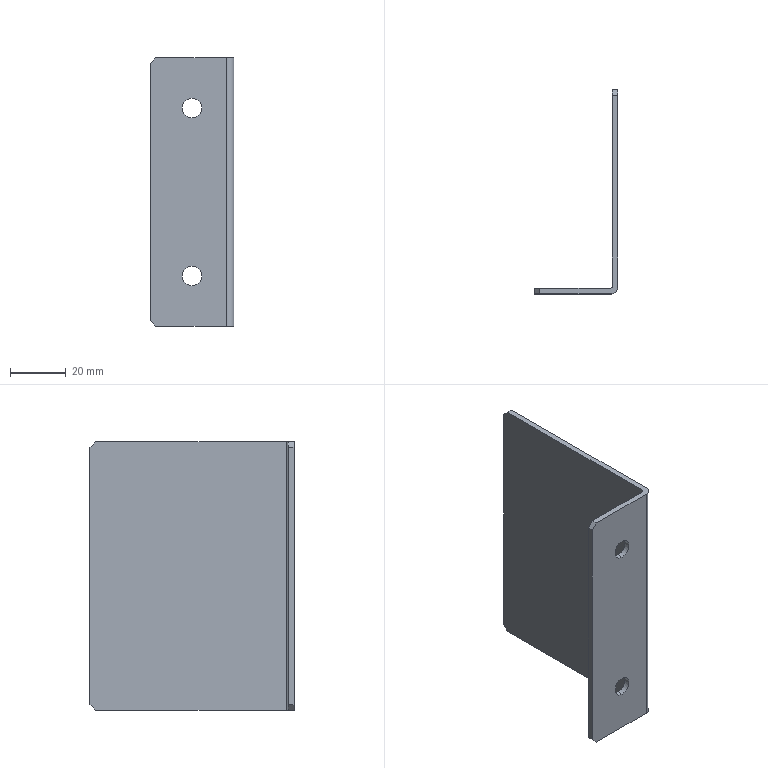Part | SolidWorks | features BaseBody 1 | 1 solid | 18 faces | box 30 x 73 x 96 mm | volume 19079 mm3 | plane 12 | cylinder 6 | commonest cylinder face diameters 7 x4 1.473 x1 5.473 x1
STEP:
#1=CARTESIAN_POINT('',(15.,0.,14.5));
#2=VERTEX_POINT('',#1);
#3=CARTESIAN_POINT('',(15.,0.,21.5));
#4=VERTEX_POINT('',#3);
#5=CARTESIAN_POINT('',(15.,0.,18.));
#6=DIRECTION('',(0.,1.,0.));
#7=DIRECTION('',(0.,0.,1.));
#8=AXIS2_PLACEMENT_3D('',#5,#6,#7);
#9=CIRCLE('',#8,3.5);
#10=EDGE_CURVE('',#2,#4,#9,.T.);
#11=ORIENTED_EDGE('',*,*,#10,.F.);
#12=CARTESIAN_POINT('',(15.,2.,14.5));
#13=VERTEX_POINT('',#12);
#14=CARTESIAN_POINT('',(15.,2.,14.5));
#15=DIRECTION('',(0.,1.,0.));
#16=VECTOR('',#15,1000.);
#17=LINE('',#14,#16);
#18=EDGE_CURVE('',#2,#13,#17,.T.);
#19=ORIENTED_EDGE('',*,*,#18,.T.);
#20=CARTESIAN_POINT('',(15.,2.,21.5));
#21=VERTEX_POINT('',#20);
#22=CARTESIAN_POINT('',(15.,2.,18.));
#23=DIRECTION('',(0.,1.,0.));
#24=DIRECTION('',(0.,0.,1.));
#25=AXIS2_PLACEMENT_3D('',#22,#23,#24);
#26=CIRCLE('',#25,3.5);
#27=EDGE_CURVE('',#13,#21,#26,.T.);
#28=ORIENTED_EDGE('',*,*,#27,.T.);
#29=CARTESIAN_POINT('',(15.,2.,21.5));
#30=DIRECTION('',(0.,1.,0.));
#31=VECTOR('',#30,1000.);
#32=LINE('',#29,#31);
#33=EDGE_CURVE('',#4,#21,#32,.T.);
#34=ORIENTED_EDGE('',*,*,#33,.F.);
#35=EDGE_LOOP('',(#11,#19,#28,#34));
#36=FACE_OUTER_BOUND('',#35,.T.);
#37=CARTESIAN_POINT('',(15.,2.,18.));
#38=DIRECTION('',(0.,1.,0.));
#39=DIRECTION('',(0.,0.,1.));
#40=AXIS2_PLACEMENT_3D('',#37,#38,#39);
#41=CYLINDRICAL_SURFACE('',#40,3.5);
#42=ADVANCED_FACE('',(#36),#41,.F.);
#43=CARTESIAN_POINT('',(15.,0.,74.5));
#44=VERTEX_POINT('',#43);
#45=CARTESIAN_POINT('',(15.,0.,81.5));
#46=VERTEX_POINT('',#45);
#47=CARTESIAN_POINT('',(15.,0.,78.));
#48=DIRECTION('',(0.,1.,0.));
#49=DIRECTION('',(0.,0.,1.));
#50=AXIS2_PLACEMENT_3D('',#47,#48,#49);
#51=CIRCLE('',#50,3.5);
#52=EDGE_CURVE('',#44,#46,#51,.T.);
#53=ORIENTED_EDGE('',*,*,#52,.F.);
#54=CARTESIAN_POINT('',(15.,2.,74.5));
#55=VERTEX_POINT('',#54);
#56=CARTESIAN_POINT('',(15.,2.,74.5));
#57=DIRECTION('',(0.,1.,0.));
#58=VECTOR('',#57,1000.);
#59=LINE('',#56,#58);
#60=EDGE_CURVE('',#44,#55,#59,.T.);
#61=ORIENTED_EDGE('',*,*,#60,.T.);
#62=CARTESIAN_POINT('',(15.,2.,81.5));
#63=VERTEX_POINT('',#62);
#64=CARTESIAN_POINT('',(15.,2.,78.));
#65=DIRECTION('',(0.,1.,0.));
#66=DIRECTION('',(0.,0.,1.));
#67=AXIS2_PLACEMENT_3D('',#64,#65,#66);
#68=CIRCLE('',#67,3.5);
#69=EDGE_CURVE('',#55,#63,#68,.T.);
#70=ORIENTED_EDGE('',*,*,#69,.T.);
#71=CARTESIAN_POINT('',(15.,2.,81.5));
#72=DIRECTION('',(0.,1.,0.));
#73=VECTOR('',#72,1000.);
#74=LINE('',#71,#73);
#75=EDGE_CURVE('',#46,#63,#74,.T.);
#76=ORIENTED_EDGE('',*,*,#75,.F.);
#77=EDGE_LOOP('',(#53,#61,#70,#76));
#78=FACE_OUTER_BOUND('',#77,.T.);
#79=CARTESIAN_POINT('',(15.,2.,78.));
#80=DIRECTION('',(0.,1.,0.));
#81=DIRECTION('',(0.,0.,1.));
#82=AXIS2_PLACEMENT_3D('',#79,#80,#81);
#83=CYLINDRICAL_SURFACE('',#82,3.5);
#84=ADVANCED_FACE('',(#78),#83,.F.);
#85=CARTESIAN_POINT('',(0.,0.,2.));
#86=VERTEX_POINT('',#85);
#87=CARTESIAN_POINT('',(2.,0.,0.));
#88=VERTEX_POINT('',#87);
#89=CARTESIAN_POINT('',(2.,0.,0.));
#90=DIRECTION('',(0.7071,0.,-0.7071));
#91=VECTOR('',#90,1000.);
#92=LINE('',#89,#91);
#93=EDGE_CURVE('',#86,#88,#92,.T.);
#94=ORIENTED_EDGE('',*,*,#93,.F.);
#95=CARTESIAN_POINT('',(0.,2.,2.));
#96=VERTEX_POINT('',#95);
#97=CARTESIAN_POINT('',(0.,0.,2.));
#98=DIRECTION('',(0.,-1.,0.));
#99=VECTOR('',#98,1000.);
#100=LINE('',#97,#99);
#101=EDGE_CURVE('',#96,#86,#100,.T.);
#102=ORIENTED_EDGE('',*,*,#101,.F.);
#103=CARTESIAN_POINT('',(2.,2.,0.));
#104=VERTEX_POINT('',#103);
#105=CARTESIAN_POINT('',(-47.,2.,49.));
#106=DIRECTION('',(-0.7071,0.,0.7071));
#107=VECTOR('',#106,1000.);
#108=LINE('',#105,#107);
#109=EDGE_CURVE('',#104,#96,#108,.T.);
#110=ORIENTED_EDGE('',*,*,#109,.F.);
#111=CARTESIAN_POINT('',(2.,2.,0.));
#112=DIRECTION('',(0.,1.,0.));
#113=VECTOR('',#112,1000.);
#114=LINE('',#111,#113);
#115=EDGE_CURVE('',#88,#104,#114,.T.);
#116=ORIENTED_EDGE('',*,*,#115,.F.);
#117=EDGE_LOOP('',(#94,#102,#110,#116));
#118=FACE_OUTER_BOUND('',#117,.T.);
#119=CARTESIAN_POINT('',(2.,2.737,0.));
#120=DIRECTION('',(-0.7071,0.,-0.7071));
#121=DIRECTION('',(-0.7071,0.,0.7071));
#122=AXIS2_PLACEMENT_3D('',#119,#120,#121);
#123=PLANE('',#122);
#124=ADVANCED_FACE('',(#118),#123,.T.);
#125=CARTESIAN_POINT('',(2.,0.,96.));
#126=VERTEX_POINT('',#125);
#127=CARTESIAN_POINT('',(0.,0.,94.));
#128=VERTEX_POINT('',#127);
#129=CARTESIAN_POINT('',(0.,0.,94.));
#130=DIRECTION('',(-0.7071,0.,-0.7071));
#131=VECTOR('',#130,1000.);
#132=LINE('',#129,#131);
#133=EDGE_CURVE('',#126,#128,#132,.T.);
#134=ORIENTED_EDGE('',*,*,#133,.F.);
#135=CARTESIAN_POINT('',(2.,2.,96.));
#136=VERTEX_POINT('',#135);
#137=CARTESIAN_POINT('',(2.,2.737,96.));
#138=DIRECTION('',(0.,-1.,0.));
#139=VECTOR('',#138,1000.);
#140=LINE('',#137,#139);
#141=EDGE_CURVE('',#136,#126,#140,.T.);
#142=ORIENTED_EDGE('',*,*,#141,.F.);
#143=CARTESIAN_POINT('',(0.,2.,94.));
#144=VERTEX_POINT('',#143);
#145=CARTESIAN_POINT('',(1.,2.,95.));
#146=DIRECTION('',(0.7071,0.,0.7071));
#147=VECTOR('',#146,1000.);
#148=LINE('',#145,#147);
#149=EDGE_CURVE('',#144,#136,#148,.T.);
#150=ORIENTED_EDGE('',*,*,#149,.F.);
#151=CARTESIAN_POINT('',(0.,0.,94.));
#152=DIRECTION('',(0.,1.,0.));
#153=VECTOR('',#152,1000.);
#154=LINE('',#151,#153);
#155=EDGE_CURVE('',#128,#144,#154,.T.);
#156=ORIENTED_EDGE('',*,*,#155,.F.);
#157=EDGE_LOOP('',(#134,#142,#150,#156));
#158=FACE_OUTER_BOUND('',#157,.T.);
#159=CARTESIAN_POINT('',(0.,0.,94.));
#160=DIRECTION('',(0.7071,0.,-0.7071));
#161=DIRECTION('',(0.,-1.,0.));
#162=AXIS2_PLACEMENT_3D('',#159,#160,#161);
#163=PLANE('',#162);
#164=ADVANCED_FACE('',(#158),#163,.F.);
#165=CARTESIAN_POINT('',(28.,73.,2.));
#166=VERTEX_POINT('',#165);
#167=CARTESIAN_POINT('',(28.,71.,0.));
#168=VERTEX_POINT('',#167);
#169=CARTESIAN_POINT('',(28.,83.5,12.5));
#170=DIRECTION('',(0.,-0.7071,-0.7071));
#171=VECTOR('',#170,1000.);
#172=LINE('',#169,#171);
#173=EDGE_CURVE('',#166,#168,#172,.T.);
#174=ORIENTED_EDGE('',*,*,#173,.F.);
#175=CARTESIAN_POINT('',(30.,73.,2.));
#176=VERTEX_POINT('',#175);
#177=CARTESIAN_POINT('',(28.,73.,2.));
#178=DIRECTION('',(-1.,0.,0.));
#179=VECTOR('',#178,1000.);
#180=LINE('',#177,#179);
#181=EDGE_CURVE('',#176,#166,#180,.T.);
#182=ORIENTED_EDGE('',*,*,#181,.F.);
#183=CARTESIAN_POINT('',(30.,71.,0.));
#184=VERTEX_POINT('',#183);
#185=CARTESIAN_POINT('',(30.,71.,0.));
#186=DIRECTION('',(0.,0.7071,0.7071));
#187=VECTOR('',#186,1000.);
#188=LINE('',#185,#187);
#189=EDGE_CURVE('',#184,#176,#188,.T.);
#190=ORIENTED_EDGE('',*,*,#189,.F.);
#191=CARTESIAN_POINT('',(27.263,71.,0.));
#192=DIRECTION('',(1.,0.,0.));
#193=VECTOR('',#192,1000.);
#194=LINE('',#191,#193);
#195=EDGE_CURVE('',#168,#184,#194,.T.);
#196=ORIENTED_EDGE('',*,*,#195,.F.);
#197=EDGE_LOOP('',(#174,#182,#190,#196));
#198=FACE_OUTER_BOUND('',#197,.T.);
#199=CARTESIAN_POINT('',(27.263,71.,0.));
#200=DIRECTION('',(0.,-0.7071,0.7071));
#201=DIRECTION('',(-1.,0.,0.));
#202=AXIS2_PLACEMENT_3D('',#199,#200,#201);
#203=PLANE('',#202);
#204=ADVANCED_FACE('',(#198),#203,.F.);
#205=CARTESIAN_POINT('',(28.,71.,96.));
#206=VERTEX_POINT('',#205);
#207=CARTESIAN_POINT('',(28.,73.,94.));
#208=VERTEX_POINT('',#207);
#209=CARTESIAN_POINT('',(28.,35.5,131.5));
#210=DIRECTION('',(0.,0.7071,-0.7071));
#211=VECTOR('',#210,1000.);
#212=LINE('',#209,#211);
#213=EDGE_CURVE('',#206,#208,#212,.T.);
#214=ORIENTED_EDGE('',*,*,#213,.F.);
#215=CARTESIAN_POINT('',(30.,71.,96.));
#216=VERTEX_POINT('',#215);
#217=CARTESIAN_POINT('',(27.263,71.,96.));
#218=DIRECTION('',(-1.,0.,0.));
#219=VECTOR('',#218,1000.);
#220=LINE('',#217,#219);
#221=EDGE_CURVE('',#216,#206,#220,.T.);
#222=ORIENTED_EDGE('',*,*,#221,.F.);
#223=CARTESIAN_POINT('',(30.,73.,94.));
#224=VERTEX_POINT('',#223);
#225=CARTESIAN_POINT('',(30.,73.,94.));
#226=DIRECTION('',(0.,-0.7071,0.7071));
#227=VECTOR('',#226,1000.);
#228=LINE('',#225,#227);
#229=EDGE_CURVE('',#224,#216,#228,.T.);
#230=ORIENTED_EDGE('',*,*,#229,.F.);
#231=CARTESIAN_POINT('',(28.,73.,94.));
#232=DIRECTION('',(1.,0.,0.));
#233=VECTOR('',#232,1000.);
#234=LINE('',#231,#233);
#235=EDGE_CURVE('',#208,#224,#234,.T.);
#236=ORIENTED_EDGE('',*,*,#235,.F.);
#237=EDGE_LOOP('',(#214,#222,#230,#236));
#238=FACE_OUTER_BOUND('',#237,.T.);
#239=CARTESIAN_POINT('',(28.,73.,94.));
#240=DIRECTION('',(0.,-0.7071,-0.7071));
#241=DIRECTION('',(0.,-0.7071,0.7071));
#242=AXIS2_PLACEMENT_3D('',#239,#240,#241);
#243=PLANE('',#242);
#244=ADVANCED_FACE('',(#238),#243,.F.);
#245=CARTESIAN_POINT('',(27.263,0.,0.));
#246=VERTEX_POINT('',#245);
#247=CARTESIAN_POINT('',(30.,2.737,0.));
#248=VERTEX_POINT('',#247);
#249=CARTESIAN_POINT('',(27.263,2.737,0.));
#250=DIRECTION('',(0.,0.,1.));
#251=DIRECTION('',(-1.,0.,0.));
#252=AXIS2_PLACEMENT_3D('',#249,#250,#251);
#253=CIRCLE('',#252,2.737);
#254=EDGE_CURVE('',#246,#248,#253,.T.);
#255=ORIENTED_EDGE('',*,*,#254,.T.);
#256=CARTESIAN_POINT('',(30.,2.737,96.));
#257=VERTEX_POINT('',#256);
#258=CARTESIAN_POINT('',(30.,2.737,96.));
#259=DIRECTION('',(0.,0.,-1.));
#260=VECTOR('',#259,1000.);
#261=LINE('',#258,#260);
#262=EDGE_CURVE('',#257,#248,#261,.T.);
#263=ORIENTED_EDGE('',*,*,#262,.F.);
#264=CARTESIAN_POINT('',(27.263,0.,96.));
#265=VERTEX_POINT('',#264);
#266=CARTESIAN_POINT('',(27.263,2.737,96.));
#267=DIRECTION('',(0.,0.,1.));
#268=DIRECTION('',(-1.,0.,0.));
#269=AXIS2_PLACEMENT_3D('',#266,#267,#268);
#270=CIRCLE('',#269,2.737);
#271=EDGE_CURVE('',#265,#257,#270,.T.);
#272=ORIENTED_EDGE('',*,*,#271,.F.);
#273=CARTESIAN_POINT('',(27.263,0.,96.));
#274=DIRECTION('',(0.,0.,-1.));
#275=VECTOR('',#274,1000.);
#276=LINE('',#273,#275);
#277=EDGE_CURVE('',#265,#246,#276,.T.);
#278=ORIENTED_EDGE('',*,*,#277,.T.);
#279=EDGE_LOOP('',(#255,#263,#272,#278));
#280=FACE_OUTER_BOUND('',#279,.T.);
#281=CARTESIAN_POINT('',(27.263,2.737,96.));
#282=DIRECTION('',(0.,0.,-1.));
#283=DIRECTION('',(-1.,0.,0.));
#284=AXIS2_PLACEMENT_3D('',#281,#282,#283);
#285=CYLINDRICAL_SURFACE('',#284,2.737);
#286=ADVANCED_FACE('',(#280),#285,.T.);
#287=CARTESIAN_POINT('',(15.,0.,78.));
#288=DIRECTION('',(0.,1.,0.));
#289=DIRECTION('',(0.,0.,1.));
#290=AXIS2_PLACEMENT_3D('',#287,#288,#289);
#291=CIRCLE('',#290,3.5);
#292=EDGE_CURVE('',#46,#44,#291,.T.);
#293=ORIENTED_EDGE('',*,*,#292,.T.);
#294=ORIENTED_EDGE('',*,*,#52,.T.);
#295=EDGE_LOOP('',(#293,#294));
#296=FACE_BOUND('',#295,.T.);
#297=CARTESIAN_POINT('',(15.,0.,18.));
#298=DIRECTION('',(0.,1.,0.));
#299=DIRECTION('',(0.,0.,1.));
#300=AXIS2_PLACEMENT_3D('',#297,#298,#299);
#301=CIRCLE('',#300,3.5);
#302=EDGE_CURVE('',#4,#2,#301,.T.);
#303=ORIENTED_EDGE('',*,*,#302,.T.);
#304=ORIENTED_EDGE('',*,*,#10,.T.);
#305=EDGE_LOOP('',(#303,#304));
#306=FACE_BOUND('',#305,.T.);
#307=CARTESIAN_POINT('',(0.,0.,96.));
#308=DIRECTION('',(1.,0.,0.));
#309=VECTOR('',#308,1000.);
#310=LINE('',#307,#309);
#311=EDGE_CURVE('',#126,#265,#310,.T.);
#312=ORIENTED_EDGE('',*,*,#311,.F.);
#313=ORIENTED_EDGE('',*,*,#133,.T.);
#314=CARTESIAN_POINT('',(0.,0.,96.));
#315=DIRECTION('',(0.,0.,-1.));
#316=VECTOR('',#315,1000.);
#317=LINE('',#314,#316);
#318=EDGE_CURVE('',#128,#86,#317,.T.);
#319=ORIENTED_EDGE('',*,*,#318,.T.);
#320=ORIENTED_EDGE('',*,*,#93,.T.);
#321=CARTESIAN_POINT('',(0.,0.,0.));
#322=DIRECTION('',(1.,0.,0.));
#323=VECTOR('',#322,1000.);
#324=LINE('',#321,#323);
#325=EDGE_CURVE('',#88,#246,#324,.T.);
#326=ORIENTED_EDGE('',*,*,#325,.T.);
#327=ORIENTED_EDGE('',*,*,#277,.F.);
#328=EDGE_LOOP('',(#312,#313,#319,#320,#326,#327));
#329=FACE_OUTER_BOUND('',#328,.T.);
#330=CARTESIAN_POINT('',(0.,0.,96.));
#331=DIRECTION('',(0.,1.,0.));
#332=DIRECTION('',(1.,0.,0.));
#333=AXIS2_PLACEMENT_3D('',#330,#331,#332);
#334=PLANE('',#333);
#335=ADVANCED_FACE('',(#296,#306,#329),#334,.F.);
#336=ORIENTED_EDGE('',*,*,#318,.F.);
#337=ORIENTED_EDGE('',*,*,#155,.T.);
#338=CARTESIAN_POINT('',(0.,2.,96.));
#339=DIRECTION('',(0.,0.,-1.));
#340=VECTOR('',#339,1000.);
#341=LINE('',#338,#340);
#342=EDGE_CURVE('',#144,#96,#341,.T.);
#343=ORIENTED_EDGE('',*,*,#342,.T.);
#344=ORIENTED_EDGE('',*,*,#101,.T.);
#345=EDGE_LOOP('',(#336,#337,#343,#344));
#346=FACE_OUTER_BOUND('',#345,.T.);
#347=CARTESIAN_POINT('',(0.,0.,96.));
#348=DIRECTION('',(-1.,0.,0.));
#349=DIRECTION('',(0.,0.,1.));
#350=AXIS2_PLACEMENT_3D('',#347,#348,#349);
#351=PLANE('',#350);
#352=ADVANCED_FACE('',(#346),#351,.T.);
#353=CARTESIAN_POINT('',(15.,2.,78.));
#354=DIRECTION('',(0.,1.,0.));
#355=DIRECTION('',(0.,0.,1.));
#356=AXIS2_PLACEMENT_3D('',#353,#354,#355);
#357=CIRCLE('',#356,3.5);
#358=EDGE_CURVE('',#63,#55,#357,.T.);
#359=ORIENTED_EDGE('',*,*,#358,.F.);
#360=ORIENTED_EDGE('',*,*,#69,.F.);
#361=EDGE_LOOP('',(#359,#360));
#362=FACE_BOUND('',#361,.T.);
#363=CARTESIAN_POINT('',(15.,2.,18.));
#364=DIRECTION('',(0.,1.,0.));
#365=DIRECTION('',(0.,0.,1.));
#366=AXIS2_PLACEMENT_3D('',#363,#364,#365);
#367=CIRCLE('',#366,3.5);
#368=EDGE_CURVE('',#21,#13,#367,.T.);
#369=ORIENTED_EDGE('',*,*,#368,.F.);
#370=ORIENTED_EDGE('',*,*,#27,.F.);
#371=EDGE_LOOP('',(#369,#370));
#372=FACE_BOUND('',#371,.T.);
#373=ORIENTED_EDGE('',*,*,#342,.F.);
#374=ORIENTED_EDGE('',*,*,#149,.T.);
#375=CARTESIAN_POINT('',(27.263,2.,96.));
#376=VERTEX_POINT('',#375);
#377=CARTESIAN_POINT('',(0.,2.,96.));
#378=DIRECTION('',(1.,0.,0.));
#379=VECTOR('',#378,1000.);
#380=LINE('',#377,#379);
#381=EDGE_CURVE('',#136,#376,#380,.T.);
#382=ORIENTED_EDGE('',*,*,#381,.T.);
#383=CARTESIAN_POINT('',(27.263,2.,0.));
#384=VERTEX_POINT('',#383);
#385=CARTESIAN_POINT('',(27.263,2.,96.));
#386=DIRECTION('',(0.,0.,-1.));
#387=VECTOR('',#386,1000.);
#388=LINE('',#385,#387);
#389=EDGE_CURVE('',#376,#384,#388,.T.);
#390=ORIENTED_EDGE('',*,*,#389,.T.);
#391=CARTESIAN_POINT('',(0.,2.,0.));
#392=DIRECTION('',(1.,0.,0.));
#393=VECTOR('',#392,1000.);
#394=LINE('',#391,#393);
#395=EDGE_CURVE('',#104,#384,#394,.T.);
#396=ORIENTED_EDGE('',*,*,#395,.F.);
#397=ORIENTED_EDGE('',*,*,#109,.T.);
#398=EDGE_LOOP('',(#373,#374,#382,#390,#396,#397));
#399=FACE_OUTER_BOUND('',#398,.T.);
#400=CARTESIAN_POINT('',(0.,2.,96.));
#401=DIRECTION('',(0.,1.,0.));
#402=DIRECTION('',(1.,0.,0.));
#403=AXIS2_PLACEMENT_3D('',#400,#401,#402);
#404=PLANE('',#403);
#405=ADVANCED_FACE('',(#362,#372,#399),#404,.T.);
#406=CARTESIAN_POINT('',(28.,2.737,0.));
#407=VERTEX_POINT('',#406);
#408=CARTESIAN_POINT('',(27.263,2.737,0.));
#409=DIRECTION('',(0.,0.,1.));
#410=DIRECTION('',(1.,0.,0.));
#411=AXIS2_PLACEMENT_3D('',#408,#409,#410);
#412=CIRCLE('',#411,0.7366);
#413=EDGE_CURVE('',#384,#407,#412,.T.);
#414=ORIENTED_EDGE('',*,*,#413,.F.);
#415=ORIENTED_EDGE('',*,*,#389,.F.);
#416=CARTESIAN_POINT('',(28.,2.737,96.));
#417=VERTEX_POINT('',#416);
#418=CARTESIAN_POINT('',(27.263,2.737,96.));
#419=DIRECTION('',(0.,0.,1.));
#420=DIRECTION('',(1.,0.,0.));
#421=AXIS2_PLACEMENT_3D('',#418,#419,#420);
#422=CIRCLE('',#421,0.7366);
#423=EDGE_CURVE('',#376,#417,#422,.T.);
#424=ORIENTED_EDGE('',*,*,#423,.T.);
#425=CARTESIAN_POINT('',(28.,2.737,96.));
#426=DIRECTION('',(0.,0.,-1.));
#427=VECTOR('',#426,1000.);
#428=LINE('',#425,#427);
#429=EDGE_CURVE('',#417,#407,#428,.T.);
#430=ORIENTED_EDGE('',*,*,#429,.T.);
#431=EDGE_LOOP('',(#414,#415,#424,#430));
#432=FACE_OUTER_BOUND('',#431,.T.);
#433=CARTESIAN_POINT('',(27.263,2.737,96.));
#434=DIRECTION('',(0.,0.,-1.));
#435=DIRECTION('',(-1.,0.,0.));
#436=AXIS2_PLACEMENT_3D('',#433,#434,#435);
#437=CYLINDRICAL_SURFACE('',#436,0.7366);
#438=ADVANCED_FACE('',(#432),#437,.F.);
#439=CARTESIAN_POINT('',(28.,0.,96.));
#440=DIRECTION('',(0.,1.,0.));
#441=VECTOR('',#440,1000.);
#442=LINE('',#439,#441);
#443=EDGE_CURVE('',#417,#206,#442,.T.);
#444=ORIENTED_EDGE('',*,*,#443,.T.);
#445=ORIENTED_EDGE('',*,*,#213,.T.);
#446=CARTESIAN_POINT('',(28.,73.,96.));
#447=DIRECTION('',(0.,0.,-1.));
#448=VECTOR('',#447,1000.);
#449=LINE('',#446,#448);
#450=EDGE_CURVE('',#208,#166,#449,.T.);
#451=ORIENTED_EDGE('',*,*,#450,.T.);
#452=ORIENTED_EDGE('',*,*,#173,.T.);
#453=CARTESIAN_POINT('',(28.,0.,0.));
#454=DIRECTION('',(0.,1.,0.));
#455=VECTOR('',#454,1000.);
#456=LINE('',#453,#455);
#457=EDGE_CURVE('',#407,#168,#456,.T.);
#458=ORIENTED_EDGE('',*,*,#457,.F.);
#459=ORIENTED_EDGE('',*,*,#429,.F.);
#460=EDGE_LOOP('',(#444,#445,#451,#452,#458,#459));
#461=FACE_OUTER_BOUND('',#460,.T.);
#462=CARTESIAN_POINT('',(28.,0.,96.));
#463=DIRECTION('',(-1.,0.,0.));
#464=DIRECTION('',(0.,0.,1.));
#465=AXIS2_PLACEMENT_3D('',#462,#463,#464);
#466=PLANE('',#465);
#467=ADVANCED_FACE('',(#461),#466,.T.);
#468=ORIENTED_EDGE('',*,*,#450,.F.);
#469=ORIENTED_EDGE('',*,*,#235,.T.);
#470=CARTESIAN_POINT('',(30.,73.,96.));
#471=DIRECTION('',(0.,0.,-1.));
#472=VECTOR('',#471,1000.);
#473=LINE('',#470,#472);
#474=EDGE_CURVE('',#224,#176,#473,.T.);
#475=ORIENTED_EDGE('',*,*,#474,.T.);
#476=ORIENTED_EDGE('',*,*,#181,.T.);
#477=EDGE_LOOP('',(#468,#469,#475,#476));
#478=FACE_OUTER_BOUND('',#477,.T.);
#479=CARTESIAN_POINT('',(28.,73.,96.));
#480=DIRECTION('',(0.,1.,0.));
#481=DIRECTION('',(1.,0.,0.));
#482=AXIS2_PLACEMENT_3D('',#479,#480,#481);
#483=PLANE('',#482);
#484=ADVANCED_FACE('',(#478),#483,.T.);
#485=ORIENTED_EDGE('',*,*,#474,.F.);
#486=ORIENTED_EDGE('',*,*,#229,.T.);
#487=CARTESIAN_POINT('',(30.,0.,96.));
#488=DIRECTION('',(0.,1.,0.));
#489=VECTOR('',#488,1000.);
#490=LINE('',#487,#489);
#491=EDGE_CURVE('',#257,#216,#490,.T.);
#492=ORIENTED_EDGE('',*,*,#491,.F.);
#493=ORIENTED_EDGE('',*,*,#262,.T.);
#494=CARTESIAN_POINT('',(30.,0.,0.));
#495=DIRECTION('',(0.,1.,0.));
#496=VECTOR('',#495,1000.);
#497=LINE('',#494,#496);
#498=EDGE_CURVE('',#248,#184,#497,.T.);
#499=ORIENTED_EDGE('',*,*,#498,.T.);
#500=ORIENTED_EDGE('',*,*,#189,.T.);
#501=EDGE_LOOP('',(#485,#486,#492,#493,#499,#500));
#502=FACE_OUTER_BOUND('',#501,.T.);
#503=CARTESIAN_POINT('',(30.,0.,96.));
#504=DIRECTION('',(-1.,0.,0.));
#505=DIRECTION('',(0.,0.,1.));
#506=AXIS2_PLACEMENT_3D('',#503,#504,#505);
#507=PLANE('',#506);
#508=ADVANCED_FACE('',(#502),#507,.F.);
#509=ORIENTED_EDGE('',*,*,#413,.T.);
#510=ORIENTED_EDGE('',*,*,#457,.T.);
#511=ORIENTED_EDGE('',*,*,#195,.T.);
#512=ORIENTED_EDGE('',*,*,#498,.F.);
#513=ORIENTED_EDGE('',*,*,#254,.F.);
#514=ORIENTED_EDGE('',*,*,#325,.F.);
#515=ORIENTED_EDGE('',*,*,#115,.T.);
#516=ORIENTED_EDGE('',*,*,#395,.T.);
#517=EDGE_LOOP('',(#509,#510,#511,#512,#513,#514,#515,#516));
#518=FACE_OUTER_BOUND('',#517,.T.);
#519=CARTESIAN_POINT('',(30.,2.737,0.));
#520=DIRECTION('',(0.,0.,-1.));
#521=DIRECTION('',(0.,-1.,0.));
#522=AXIS2_PLACEMENT_3D('',#519,#520,#521);
#523=PLANE('',#522);
#524=ADVANCED_FACE('',(#518),#523,.T.);
#525=ORIENTED_EDGE('',*,*,#423,.F.);
#526=ORIENTED_EDGE('',*,*,#381,.F.);
#527=ORIENTED_EDGE('',*,*,#141,.T.);
#528=ORIENTED_EDGE('',*,*,#311,.T.);
#529=ORIENTED_EDGE('',*,*,#271,.T.);
#530=ORIENTED_EDGE('',*,*,#491,.T.);
#531=ORIENTED_EDGE('',*,*,#221,.T.);
#532=ORIENTED_EDGE('',*,*,#443,.F.);
#533=EDGE_LOOP('',(#525,#526,#527,#528,#529,#530,#531,#532));
#534=FACE_OUTER_BOUND('',#533,.T.);
#535=CARTESIAN_POINT('',(27.263,0.,96.));
#536=DIRECTION('',(0.,0.,1.));
#537=DIRECTION('',(1.,0.,0.));
#538=AXIS2_PLACEMENT_3D('',#535,#536,#537);
#539=PLANE('',#538);
#540=ADVANCED_FACE('',(#534),#539,.T.);
#541=ORIENTED_EDGE('',*,*,#60,.F.);
#542=ORIENTED_EDGE('',*,*,#292,.F.);
#543=ORIENTED_EDGE('',*,*,#75,.T.);
#544=ORIENTED_EDGE('',*,*,#358,.T.);
#545=EDGE_LOOP('',(#541,#542,#543,#544));
#546=FACE_OUTER_BOUND('',#545,.T.);
#547=CARTESIAN_POINT('',(15.,2.,78.));
#548=DIRECTION('',(0.,1.,0.));
#549=DIRECTION('',(0.,0.,1.));
#550=AXIS2_PLACEMENT_3D('',#547,#548,#549);
#551=CYLINDRICAL_SURFACE('',#550,3.5);
#552=ADVANCED_FACE('',(#546),#551,.F.);
#553=ORIENTED_EDGE('',*,*,#18,.F.);
#554=ORIENTED_EDGE('',*,*,#302,.F.);
#555=ORIENTED_EDGE('',*,*,#33,.T.);
#556=ORIENTED_EDGE('',*,*,#368,.T.);
#557=EDGE_LOOP('',(#553,#554,#555,#556));
#558=FACE_OUTER_BOUND('',#557,.T.);
#559=CARTESIAN_POINT('',(15.,2.,18.));
#560=DIRECTION('',(0.,1.,0.));
#561=DIRECTION('',(0.,0.,1.));
#562=AXIS2_PLACEMENT_3D('',#559,#560,#561);
#563=CYLINDRICAL_SURFACE('',#562,3.5);
#564=ADVANCED_FACE('',(#558),#563,.F.);
#565=CLOSED_SHELL('',(#42,#84,#124,#164,#204,#244,#286,#335,#352,#405,#438,#467,#484,#508,#524,#540,#552,#564));
#566=MANIFOLD_SOLID_BREP('',#565);
#567=CARTESIAN_POINT('',(0.,0.,0.));
#568=DIRECTION('',(0.,0.,1.));
#569=DIRECTION('',(1.,0.,0.));
#570=AXIS2_PLACEMENT_3D('',#567,#568,#569);
#571=(LENGTH_UNIT()NAMED_UNIT(*)SI_UNIT(.MILLI.,.METRE.));
#572=UNCERTAINTY_MEASURE_WITH_UNIT(LENGTH_MEASURE(0.00001),#571,'','');
#573=(NAMED_UNIT(*)PLANE_ANGLE_UNIT()SI_UNIT($,.RADIAN.));
#574=(NAMED_UNIT(*)SI_UNIT($,.STERADIAN.)SOLID_ANGLE_UNIT());
#575=(GEOMETRIC_REPRESENTATION_CONTEXT(3)GLOBAL_UNCERTAINTY_ASSIGNED_CONTEXT((#572))GLOBAL_UNIT_ASSIGNED_CONTEXT((#571,#573,#574))REPRESENTATION_CONTEXT('',''));
#576=ADVANCED_BREP_SHAPE_REPRESENTATION('',(#566,#570),#575);